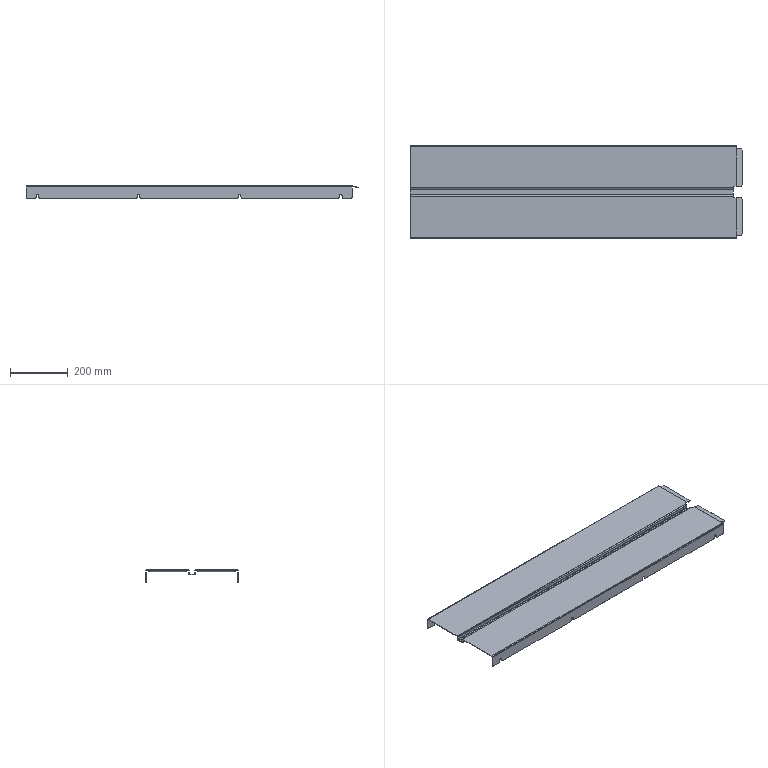Part | STEP file | BELT.PLATE.2.stp | 1 solid | 111 faces | box 1150 x 320 x 43 mm | volume 966060 mm3 | spline 52 | cylinder 33 | plane 26 | commonest cylinder face diameters 10 x15 8 x8 4 x6 9 x4